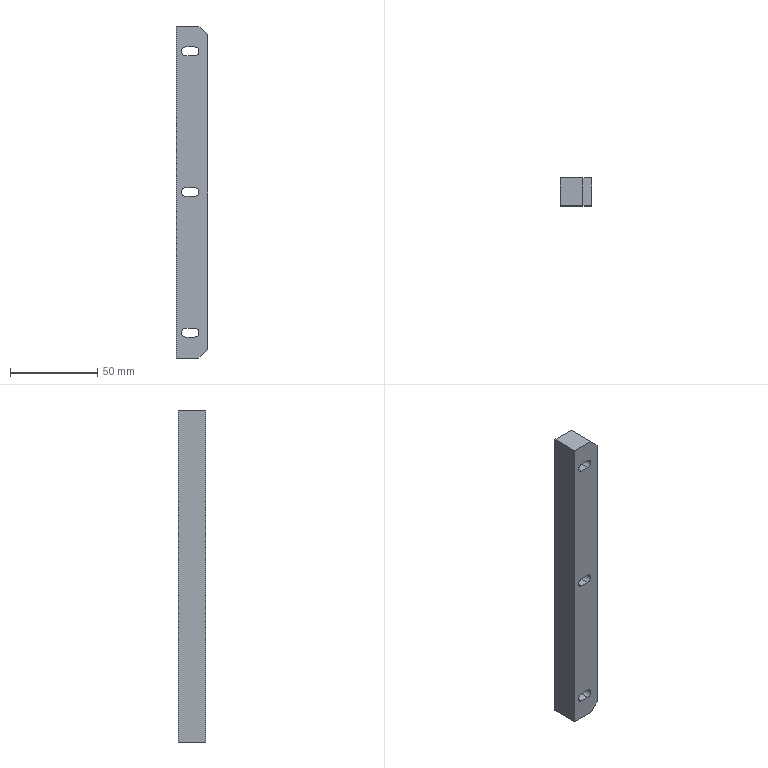Part | SolidWorks | features Chamfer 1, Extrusion 1, ICE 1 | 1 solid | 23 faces | box 18 x 16 x 190 mm | volume 52178 mm3 | plane 14 | cylinder 9 | commonest cylinder face diameters 5 x9
STEP:
#1=CARTESIAN_POINT('',(10.5,16.,83.));
#2=VERTEX_POINT('',#1);
#3=CARTESIAN_POINT('',(13.,16.,80.5));
#4=VERTEX_POINT('',#3);
#5=CARTESIAN_POINT('',(10.5,16.,80.5));
#6=DIRECTION('',(0.,1.,0.));
#7=DIRECTION('',(0.,0.,-1.));
#8=AXIS2_PLACEMENT_3D('',#5,#6,#7);
#9=CIRCLE('',#8,2.5);
#10=EDGE_CURVE('',#2,#4,#9,.T.);
#11=ORIENTED_EDGE('',*,*,#10,.T.);
#12=CARTESIAN_POINT('',(13.,0.,80.5));
#13=VERTEX_POINT('',#12);
#14=CARTESIAN_POINT('',(13.,16.001,80.5));
#15=DIRECTION('',(0.,-1.,0.));
#16=VECTOR('',#15,1000.);
#17=LINE('',#14,#16);
#18=EDGE_CURVE('',#4,#13,#17,.T.);
#19=ORIENTED_EDGE('',*,*,#18,.T.);
#20=CARTESIAN_POINT('',(10.5,0.,83.));
#21=VERTEX_POINT('',#20);
#22=CARTESIAN_POINT('',(10.5,0.,80.5));
#23=DIRECTION('',(0.,-1.,0.));
#24=DIRECTION('',(1.,0.,0.));
#25=AXIS2_PLACEMENT_3D('',#22,#23,#24);
#26=CIRCLE('',#25,2.5);
#27=EDGE_CURVE('',#13,#21,#26,.T.);
#28=ORIENTED_EDGE('',*,*,#27,.T.);
#29=CARTESIAN_POINT('',(10.5,16.001,83.));
#30=DIRECTION('',(0.,-1.,0.));
#31=VECTOR('',#30,1000.);
#32=LINE('',#29,#31);
#33=EDGE_CURVE('',#2,#21,#32,.T.);
#34=ORIENTED_EDGE('',*,*,#33,.F.);
#35=EDGE_LOOP('',(#11,#19,#28,#34));
#36=FACE_OUTER_BOUND('',#35,.T.);
#37=CARTESIAN_POINT('',(10.5,16.001,80.5));
#38=DIRECTION('',(0.,-1.,0.));
#39=DIRECTION('',(1.,0.,0.));
#40=AXIS2_PLACEMENT_3D('',#37,#38,#39);
#41=CYLINDRICAL_SURFACE('',#40,2.5);
#42=ADVANCED_FACE('',(#36),#41,.F.);
#43=CARTESIAN_POINT('',(10.5,16.,2.5));
#44=VERTEX_POINT('',#43);
#45=CARTESIAN_POINT('',(13.,16.,0.));
#46=VERTEX_POINT('',#45);
#47=CARTESIAN_POINT('',(10.5,16.,0.));
#48=DIRECTION('',(0.,1.,0.));
#49=DIRECTION('',(0.,0.,-1.));
#50=AXIS2_PLACEMENT_3D('',#47,#48,#49);
#51=CIRCLE('',#50,2.5);
#52=EDGE_CURVE('',#44,#46,#51,.T.);
#53=ORIENTED_EDGE('',*,*,#52,.T.);
#54=CARTESIAN_POINT('',(13.,0.,0.));
#55=VERTEX_POINT('',#54);
#56=CARTESIAN_POINT('',(13.,16.001,0.));
#57=DIRECTION('',(0.,-1.,0.));
#58=VECTOR('',#57,1000.);
#59=LINE('',#56,#58);
#60=EDGE_CURVE('',#46,#55,#59,.T.);
#61=ORIENTED_EDGE('',*,*,#60,.T.);
#62=CARTESIAN_POINT('',(10.5,0.,2.5));
#63=VERTEX_POINT('',#62);
#64=CARTESIAN_POINT('',(10.5,0.,0.));
#65=DIRECTION('',(0.,-1.,0.));
#66=DIRECTION('',(1.,0.,0.));
#67=AXIS2_PLACEMENT_3D('',#64,#65,#66);
#68=CIRCLE('',#67,2.5);
#69=EDGE_CURVE('',#55,#63,#68,.T.);
#70=ORIENTED_EDGE('',*,*,#69,.T.);
#71=CARTESIAN_POINT('',(10.5,16.001,2.5));
#72=DIRECTION('',(0.,-1.,0.));
#73=VECTOR('',#72,1000.);
#74=LINE('',#71,#73);
#75=EDGE_CURVE('',#44,#63,#74,.T.);
#76=ORIENTED_EDGE('',*,*,#75,.F.);
#77=EDGE_LOOP('',(#53,#61,#70,#76));
#78=FACE_OUTER_BOUND('',#77,.T.);
#79=CARTESIAN_POINT('',(10.5,16.001,0.));
#80=DIRECTION('',(0.,-1.,0.));
#81=DIRECTION('',(1.,0.,0.));
#82=AXIS2_PLACEMENT_3D('',#79,#80,#81);
#83=CYLINDRICAL_SURFACE('',#82,2.5);
#84=ADVANCED_FACE('',(#78),#83,.F.);
#85=CARTESIAN_POINT('',(10.5,16.,-78.));
#86=VERTEX_POINT('',#85);
#87=CARTESIAN_POINT('',(13.,16.,-80.5));
#88=VERTEX_POINT('',#87);
#89=CARTESIAN_POINT('',(10.5,16.,-80.5));
#90=DIRECTION('',(0.,1.,0.));
#91=DIRECTION('',(0.,0.,-1.));
#92=AXIS2_PLACEMENT_3D('',#89,#90,#91);
#93=CIRCLE('',#92,2.5);
#94=EDGE_CURVE('',#86,#88,#93,.T.);
#95=ORIENTED_EDGE('',*,*,#94,.T.);
#96=CARTESIAN_POINT('',(13.,0.,-80.5));
#97=VERTEX_POINT('',#96);
#98=CARTESIAN_POINT('',(13.,16.001,-80.5));
#99=DIRECTION('',(0.,-1.,0.));
#100=VECTOR('',#99,1000.);
#101=LINE('',#98,#100);
#102=EDGE_CURVE('',#88,#97,#101,.T.);
#103=ORIENTED_EDGE('',*,*,#102,.T.);
#104=CARTESIAN_POINT('',(10.5,0.,-78.));
#105=VERTEX_POINT('',#104);
#106=CARTESIAN_POINT('',(10.5,0.,-80.5));
#107=DIRECTION('',(0.,-1.,0.));
#108=DIRECTION('',(-1.,0.,0.));
#109=AXIS2_PLACEMENT_3D('',#106,#107,#108);
#110=CIRCLE('',#109,2.5);
#111=EDGE_CURVE('',#97,#105,#110,.T.);
#112=ORIENTED_EDGE('',*,*,#111,.T.);
#113=CARTESIAN_POINT('',(10.5,16.001,-78.));
#114=DIRECTION('',(0.,-1.,0.));
#115=VECTOR('',#114,1000.);
#116=LINE('',#113,#115);
#117=EDGE_CURVE('',#86,#105,#116,.T.);
#118=ORIENTED_EDGE('',*,*,#117,.F.);
#119=EDGE_LOOP('',(#95,#103,#112,#118));
#120=FACE_OUTER_BOUND('',#119,.T.);
#121=CARTESIAN_POINT('',(10.5,16.001,-80.5));
#122=DIRECTION('',(0.,-1.,0.));
#123=DIRECTION('',(1.,0.,0.));
#124=AXIS2_PLACEMENT_3D('',#121,#122,#123);
#125=CYLINDRICAL_SURFACE('',#124,2.5);
#126=ADVANCED_FACE('',(#120),#125,.F.);
#127=CARTESIAN_POINT('',(5.5,0.,78.));
#128=VERTEX_POINT('',#127);
#129=CARTESIAN_POINT('',(10.5,0.,78.));
#130=VERTEX_POINT('',#129);
#131=CARTESIAN_POINT('',(5.5,0.,78.));
#132=DIRECTION('',(1.,0.,0.));
#133=VECTOR('',#132,1000.);
#134=LINE('',#131,#133);
#135=EDGE_CURVE('',#128,#130,#134,.T.);
#136=ORIENTED_EDGE('',*,*,#135,.F.);
#137=CARTESIAN_POINT('',(5.5,0.,83.));
#138=VERTEX_POINT('',#137);
#139=CARTESIAN_POINT('',(5.5,0.,80.5));
#140=DIRECTION('',(0.,-1.,0.));
#141=DIRECTION('',(1.,0.,0.));
#142=AXIS2_PLACEMENT_3D('',#139,#140,#141);
#143=CIRCLE('',#142,2.5);
#144=EDGE_CURVE('',#138,#128,#143,.T.);
#145=ORIENTED_EDGE('',*,*,#144,.F.);
#146=CARTESIAN_POINT('',(5.5,0.,83.));
#147=DIRECTION('',(-1.,0.,0.));
#148=VECTOR('',#147,1000.);
#149=LINE('',#146,#148);
#150=EDGE_CURVE('',#21,#138,#149,.T.);
#151=ORIENTED_EDGE('',*,*,#150,.F.);
#152=ORIENTED_EDGE('',*,*,#27,.F.);
#153=CARTESIAN_POINT('',(10.5,0.,80.5));
#154=DIRECTION('',(0.,-1.,0.));
#155=DIRECTION('',(1.,0.,0.));
#156=AXIS2_PLACEMENT_3D('',#153,#154,#155);
#157=CIRCLE('',#156,2.5);
#158=EDGE_CURVE('',#130,#13,#157,.T.);
#159=ORIENTED_EDGE('',*,*,#158,.F.);
#160=EDGE_LOOP('',(#136,#145,#151,#152,#159));
#161=FACE_BOUND('',#160,.T.);
#162=CARTESIAN_POINT('',(5.5,0.,-2.5));
#163=VERTEX_POINT('',#162);
#164=CARTESIAN_POINT('',(10.5,0.,-2.5));
#165=VERTEX_POINT('',#164);
#166=CARTESIAN_POINT('',(5.5,0.,-2.5));
#167=DIRECTION('',(1.,0.,0.));
#168=VECTOR('',#167,1000.);
#169=LINE('',#166,#168);
#170=EDGE_CURVE('',#163,#165,#169,.T.);
#171=ORIENTED_EDGE('',*,*,#170,.F.);
#172=CARTESIAN_POINT('',(5.5,0.,2.5));
#173=VERTEX_POINT('',#172);
#174=CARTESIAN_POINT('',(5.5,0.,0.));
#175=DIRECTION('',(0.,-1.,0.));
#176=DIRECTION('',(1.,0.,0.));
#177=AXIS2_PLACEMENT_3D('',#174,#175,#176);
#178=CIRCLE('',#177,2.5);
#179=EDGE_CURVE('',#173,#163,#178,.T.);
#180=ORIENTED_EDGE('',*,*,#179,.F.);
#181=CARTESIAN_POINT('',(5.5,0.,2.5));
#182=DIRECTION('',(-1.,0.,0.));
#183=VECTOR('',#182,1000.);
#184=LINE('',#181,#183);
#185=EDGE_CURVE('',#63,#173,#184,.T.);
#186=ORIENTED_EDGE('',*,*,#185,.F.);
#187=ORIENTED_EDGE('',*,*,#69,.F.);
#188=CARTESIAN_POINT('',(10.5,0.,0.));
#189=DIRECTION('',(0.,-1.,0.));
#190=DIRECTION('',(1.,0.,0.));
#191=AXIS2_PLACEMENT_3D('',#188,#189,#190);
#192=CIRCLE('',#191,2.5);
#193=EDGE_CURVE('',#165,#55,#192,.T.);
#194=ORIENTED_EDGE('',*,*,#193,.F.);
#195=EDGE_LOOP('',(#171,#180,#186,#187,#194));
#196=FACE_BOUND('',#195,.T.);
#197=CARTESIAN_POINT('',(5.5,0.,-83.));
#198=VERTEX_POINT('',#197);
#199=CARTESIAN_POINT('',(10.5,0.,-83.));
#200=VERTEX_POINT('',#199);
#201=CARTESIAN_POINT('',(5.5,0.,-83.));
#202=DIRECTION('',(1.,0.,0.));
#203=VECTOR('',#202,1000.);
#204=LINE('',#201,#203);
#205=EDGE_CURVE('',#198,#200,#204,.T.);
#206=ORIENTED_EDGE('',*,*,#205,.F.);
#207=CARTESIAN_POINT('',(5.5,0.,-78.));
#208=VERTEX_POINT('',#207);
#209=CARTESIAN_POINT('',(5.5,0.,-80.5));
#210=DIRECTION('',(0.,-1.,0.));
#211=DIRECTION('',(-1.,0.,0.));
#212=AXIS2_PLACEMENT_3D('',#209,#210,#211);
#213=CIRCLE('',#212,2.5);
#214=EDGE_CURVE('',#208,#198,#213,.T.);
#215=ORIENTED_EDGE('',*,*,#214,.F.);
#216=CARTESIAN_POINT('',(5.5,0.,-78.));
#217=DIRECTION('',(-1.,0.,0.));
#218=VECTOR('',#217,1000.);
#219=LINE('',#216,#218);
#220=EDGE_CURVE('',#105,#208,#219,.T.);
#221=ORIENTED_EDGE('',*,*,#220,.F.);
#222=ORIENTED_EDGE('',*,*,#111,.F.);
#223=CARTESIAN_POINT('',(10.5,0.,-80.5));
#224=DIRECTION('',(0.,-1.,0.));
#225=DIRECTION('',(-1.,0.,0.));
#226=AXIS2_PLACEMENT_3D('',#223,#224,#225);
#227=CIRCLE('',#226,2.5);
#228=EDGE_CURVE('',#200,#97,#227,.T.);
#229=ORIENTED_EDGE('',*,*,#228,.F.);
#230=EDGE_LOOP('',(#206,#215,#221,#222,#229));
#231=FACE_BOUND('',#230,.T.);
#232=CARTESIAN_POINT('',(0.,0.,-95.));
#233=VERTEX_POINT('',#232);
#234=CARTESIAN_POINT('',(13.,0.,-95.));
#235=VERTEX_POINT('',#234);
#236=CARTESIAN_POINT('',(18.,0.,-95.));
#237=DIRECTION('',(1.,0.,0.));
#238=VECTOR('',#237,1000.);
#239=LINE('',#236,#238);
#240=EDGE_CURVE('',#233,#235,#239,.T.);
#241=ORIENTED_EDGE('',*,*,#240,.T.);
#242=CARTESIAN_POINT('',(18.,0.,-90.));
#243=VERTEX_POINT('',#242);
#244=CARTESIAN_POINT('',(18.,0.,-90.));
#245=DIRECTION('',(0.7071,0.,0.7071));
#246=VECTOR('',#245,1000.);
#247=LINE('',#244,#246);
#248=EDGE_CURVE('',#235,#243,#247,.T.);
#249=ORIENTED_EDGE('',*,*,#248,.T.);
#250=CARTESIAN_POINT('',(18.,0.,90.));
#251=VERTEX_POINT('',#250);
#252=CARTESIAN_POINT('',(18.,0.,95.));
#253=DIRECTION('',(0.,0.,-1.));
#254=VECTOR('',#253,1000.);
#255=LINE('',#252,#254);
#256=EDGE_CURVE('',#251,#243,#255,.T.);
#257=ORIENTED_EDGE('',*,*,#256,.F.);
#258=CARTESIAN_POINT('',(13.,0.,95.));
#259=VERTEX_POINT('',#258);
#260=CARTESIAN_POINT('',(13.,0.,95.));
#261=DIRECTION('',(-0.7071,0.,0.7071));
#262=VECTOR('',#261,1000.);
#263=LINE('',#260,#262);
#264=EDGE_CURVE('',#251,#259,#263,.T.);
#265=ORIENTED_EDGE('',*,*,#264,.T.);
#266=CARTESIAN_POINT('',(0.,0.,95.));
#267=VERTEX_POINT('',#266);
#268=CARTESIAN_POINT('',(18.,0.,95.));
#269=DIRECTION('',(1.,0.,0.));
#270=VECTOR('',#269,1000.);
#271=LINE('',#268,#270);
#272=EDGE_CURVE('',#267,#259,#271,.T.);
#273=ORIENTED_EDGE('',*,*,#272,.F.);
#274=CARTESIAN_POINT('',(0.,0.,95.));
#275=DIRECTION('',(0.,0.,-1.));
#276=VECTOR('',#275,1000.);
#277=LINE('',#274,#276);
#278=EDGE_CURVE('',#267,#233,#277,.T.);
#279=ORIENTED_EDGE('',*,*,#278,.T.);
#280=EDGE_LOOP('',(#241,#249,#257,#265,#273,#279));
#281=FACE_OUTER_BOUND('',#280,.T.);
#282=CARTESIAN_POINT('',(18.,0.,95.));
#283=DIRECTION('',(0.,1.,0.));
#284=DIRECTION('',(-1.,0.,0.));
#285=AXIS2_PLACEMENT_3D('',#282,#283,#284);
#286=PLANE('',#285);
#287=ADVANCED_FACE('',(#161,#196,#231,#281),#286,.F.);
#288=ORIENTED_EDGE('',*,*,#256,.T.);
#289=CARTESIAN_POINT('',(18.,16.,-90.));
#290=VERTEX_POINT('',#289);
#291=CARTESIAN_POINT('',(18.,16.,-90.));
#292=DIRECTION('',(0.,1.,0.));
#293=VECTOR('',#292,1000.);
#294=LINE('',#291,#293);
#295=EDGE_CURVE('',#243,#290,#294,.T.);
#296=ORIENTED_EDGE('',*,*,#295,.T.);
#297=CARTESIAN_POINT('',(18.,16.,90.));
#298=VERTEX_POINT('',#297);
#299=CARTESIAN_POINT('',(18.,16.,95.));
#300=DIRECTION('',(0.,0.,-1.));
#301=VECTOR('',#300,1000.);
#302=LINE('',#299,#301);
#303=EDGE_CURVE('',#298,#290,#302,.T.);
#304=ORIENTED_EDGE('',*,*,#303,.F.);
#305=CARTESIAN_POINT('',(18.,16.,90.));
#306=DIRECTION('',(0.,-1.,0.));
#307=VECTOR('',#306,1000.);
#308=LINE('',#305,#307);
#309=EDGE_CURVE('',#298,#251,#308,.T.);
#310=ORIENTED_EDGE('',*,*,#309,.T.);
#311=EDGE_LOOP('',(#288,#296,#304,#310));
#312=FACE_OUTER_BOUND('',#311,.T.);
#313=CARTESIAN_POINT('',(18.,16.,95.));
#314=DIRECTION('',(-1.,0.,0.));
#315=DIRECTION('',(0.,-1.,0.));
#316=AXIS2_PLACEMENT_3D('',#313,#314,#315);
#317=PLANE('',#316);
#318=ADVANCED_FACE('',(#312),#317,.F.);
#319=CARTESIAN_POINT('',(5.5,16.,83.));
#320=VERTEX_POINT('',#319);
#321=CARTESIAN_POINT('',(5.5,16.,83.));
#322=DIRECTION('',(1.,0.,0.));
#323=VECTOR('',#322,1000.);
#324=LINE('',#321,#323);
#325=EDGE_CURVE('',#320,#2,#324,.T.);
#326=ORIENTED_EDGE('',*,*,#325,.F.);
#327=CARTESIAN_POINT('',(5.5,16.,78.));
#328=VERTEX_POINT('',#327);
#329=CARTESIAN_POINT('',(5.5,16.,80.5));
#330=DIRECTION('',(0.,1.,0.));
#331=DIRECTION('',(0.,0.,-1.));
#332=AXIS2_PLACEMENT_3D('',#329,#330,#331);
#333=CIRCLE('',#332,2.5);
#334=EDGE_CURVE('',#328,#320,#333,.T.);
#335=ORIENTED_EDGE('',*,*,#334,.F.);
#336=CARTESIAN_POINT('',(10.5,16.,78.));
#337=VERTEX_POINT('',#336);
#338=CARTESIAN_POINT('',(5.5,16.,78.));
#339=DIRECTION('',(-1.,0.,0.));
#340=VECTOR('',#339,1000.);
#341=LINE('',#338,#340);
#342=EDGE_CURVE('',#337,#328,#341,.T.);
#343=ORIENTED_EDGE('',*,*,#342,.F.);
#344=CARTESIAN_POINT('',(10.5,16.,80.5));
#345=DIRECTION('',(0.,1.,0.));
#346=DIRECTION('',(0.,0.,-1.));
#347=AXIS2_PLACEMENT_3D('',#344,#345,#346);
#348=CIRCLE('',#347,2.5);
#349=EDGE_CURVE('',#4,#337,#348,.T.);
#350=ORIENTED_EDGE('',*,*,#349,.F.);
#351=ORIENTED_EDGE('',*,*,#10,.F.);
#352=EDGE_LOOP('',(#326,#335,#343,#350,#351));
#353=FACE_BOUND('',#352,.T.);
#354=CARTESIAN_POINT('',(5.5,16.,2.5));
#355=VERTEX_POINT('',#354);
#356=CARTESIAN_POINT('',(5.5,16.,2.5));
#357=DIRECTION('',(1.,0.,0.));
#358=VECTOR('',#357,1000.);
#359=LINE('',#356,#358);
#360=EDGE_CURVE('',#355,#44,#359,.T.);
#361=ORIENTED_EDGE('',*,*,#360,.F.);
#362=CARTESIAN_POINT('',(5.5,16.,-2.5));
#363=VERTEX_POINT('',#362);
#364=CARTESIAN_POINT('',(5.5,16.,0.));
#365=DIRECTION('',(0.,1.,0.));
#366=DIRECTION('',(0.,0.,-1.));
#367=AXIS2_PLACEMENT_3D('',#364,#365,#366);
#368=CIRCLE('',#367,2.5);
#369=EDGE_CURVE('',#363,#355,#368,.T.);
#370=ORIENTED_EDGE('',*,*,#369,.F.);
#371=CARTESIAN_POINT('',(10.5,16.,-2.5));
#372=VERTEX_POINT('',#371);
#373=CARTESIAN_POINT('',(5.5,16.,-2.5));
#374=DIRECTION('',(-1.,0.,0.));
#375=VECTOR('',#374,1000.);
#376=LINE('',#373,#375);
#377=EDGE_CURVE('',#372,#363,#376,.T.);
#378=ORIENTED_EDGE('',*,*,#377,.F.);
#379=CARTESIAN_POINT('',(10.5,16.,0.));
#380=DIRECTION('',(0.,1.,0.));
#381=DIRECTION('',(0.,0.,-1.));
#382=AXIS2_PLACEMENT_3D('',#379,#380,#381);
#383=CIRCLE('',#382,2.5);
#384=EDGE_CURVE('',#46,#372,#383,.T.);
#385=ORIENTED_EDGE('',*,*,#384,.F.);
#386=ORIENTED_EDGE('',*,*,#52,.F.);
#387=EDGE_LOOP('',(#361,#370,#378,#385,#386));
#388=FACE_BOUND('',#387,.T.);
#389=CARTESIAN_POINT('',(5.5,16.,-78.));
#390=VERTEX_POINT('',#389);
#391=CARTESIAN_POINT('',(5.5,16.,-78.));
#392=DIRECTION('',(1.,0.,0.));
#393=VECTOR('',#392,1000.);
#394=LINE('',#391,#393);
#395=EDGE_CURVE('',#390,#86,#394,.T.);
#396=ORIENTED_EDGE('',*,*,#395,.F.);
#397=CARTESIAN_POINT('',(5.5,16.,-83.));
#398=VERTEX_POINT('',#397);
#399=CARTESIAN_POINT('',(5.5,16.,-80.5));
#400=DIRECTION('',(0.,1.,0.));
#401=DIRECTION('',(0.,0.,-1.));
#402=AXIS2_PLACEMENT_3D('',#399,#400,#401);
#403=CIRCLE('',#402,2.5);
#404=EDGE_CURVE('',#398,#390,#403,.T.);
#405=ORIENTED_EDGE('',*,*,#404,.F.);
#406=CARTESIAN_POINT('',(10.5,16.,-83.));
#407=VERTEX_POINT('',#406);
#408=CARTESIAN_POINT('',(5.5,16.,-83.));
#409=DIRECTION('',(-1.,0.,0.));
#410=VECTOR('',#409,1000.);
#411=LINE('',#408,#410);
#412=EDGE_CURVE('',#407,#398,#411,.T.);
#413=ORIENTED_EDGE('',*,*,#412,.F.);
#414=CARTESIAN_POINT('',(10.5,16.,-80.5));
#415=DIRECTION('',(0.,1.,0.));
#416=DIRECTION('',(0.,0.,-1.));
#417=AXIS2_PLACEMENT_3D('',#414,#415,#416);
#418=CIRCLE('',#417,2.5);
#419=EDGE_CURVE('',#88,#407,#418,.T.);
#420=ORIENTED_EDGE('',*,*,#419,.F.);
#421=ORIENTED_EDGE('',*,*,#94,.F.);
#422=EDGE_LOOP('',(#396,#405,#413,#420,#421));
#423=FACE_BOUND('',#422,.T.);
#424=ORIENTED_EDGE('',*,*,#303,.T.);
#425=CARTESIAN_POINT('',(13.,16.,-95.));
#426=VERTEX_POINT('',#425);
#427=CARTESIAN_POINT('',(18.,16.,-90.));
#428=DIRECTION('',(-0.7071,0.,-0.7071));
#429=VECTOR('',#428,1000.);
#430=LINE('',#427,#429);
#431=EDGE_CURVE('',#290,#426,#430,.T.);
#432=ORIENTED_EDGE('',*,*,#431,.T.);
#433=CARTESIAN_POINT('',(0.,16.,-95.));
#434=VERTEX_POINT('',#433);
#435=CARTESIAN_POINT('',(0.,16.,-95.));
#436=DIRECTION('',(-1.,0.,0.));
#437=VECTOR('',#436,1000.);
#438=LINE('',#435,#437);
#439=EDGE_CURVE('',#426,#434,#438,.T.);
#440=ORIENTED_EDGE('',*,*,#439,.T.);
#441=CARTESIAN_POINT('',(0.,16.,95.));
#442=VERTEX_POINT('',#441);
#443=CARTESIAN_POINT('',(0.,16.,95.));
#444=DIRECTION('',(0.,0.,-1.));
#445=VECTOR('',#444,1000.);
#446=LINE('',#443,#445);
#447=EDGE_CURVE('',#442,#434,#446,.T.);
#448=ORIENTED_EDGE('',*,*,#447,.F.);
#449=CARTESIAN_POINT('',(13.,16.,95.));
#450=VERTEX_POINT('',#449);
#451=CARTESIAN_POINT('',(0.,16.,95.));
#452=DIRECTION('',(-1.,0.,0.));
#453=VECTOR('',#452,1000.);
#454=LINE('',#451,#453);
#455=EDGE_CURVE('',#450,#442,#454,.T.);
#456=ORIENTED_EDGE('',*,*,#455,.F.);
#457=CARTESIAN_POINT('',(13.,16.,95.));
#458=DIRECTION('',(0.7071,0.,-0.7071));
#459=VECTOR('',#458,1000.);
#460=LINE('',#457,#459);
#461=EDGE_CURVE('',#450,#298,#460,.T.);
#462=ORIENTED_EDGE('',*,*,#461,.T.);
#463=EDGE_LOOP('',(#424,#432,#440,#448,#456,#462));
#464=FACE_OUTER_BOUND('',#463,.T.);
#465=CARTESIAN_POINT('',(0.,16.,95.));
#466=DIRECTION('',(0.,-1.,0.));
#467=DIRECTION('',(0.,0.,-1.));
#468=AXIS2_PLACEMENT_3D('',#465,#466,#467);
#469=PLANE('',#468);
#470=ADVANCED_FACE('',(#353,#388,#423,#464),#469,.F.);
#471=CARTESIAN_POINT('',(0.,0.,-95.));
#472=DIRECTION('',(0.,-1.,0.));
#473=VECTOR('',#472,1000.);
#474=LINE('',#471,#473);
#475=EDGE_CURVE('',#434,#233,#474,.T.);
#476=ORIENTED_EDGE('',*,*,#475,.T.);
#477=ORIENTED_EDGE('',*,*,#278,.F.);
#478=CARTESIAN_POINT('',(0.,0.,95.));
#479=DIRECTION('',(0.,-1.,0.));
#480=VECTOR('',#479,1000.);
#481=LINE('',#478,#480);
#482=EDGE_CURVE('',#442,#267,#481,.T.);
#483=ORIENTED_EDGE('',*,*,#482,.F.);
#484=ORIENTED_EDGE('',*,*,#447,.T.);
#485=EDGE_LOOP('',(#476,#477,#483,#484));
#486=FACE_OUTER_BOUND('',#485,.T.);
#487=CARTESIAN_POINT('',(0.,0.,95.));
#488=DIRECTION('',(1.,0.,0.));
#489=DIRECTION('',(0.,0.,-1.));
#490=AXIS2_PLACEMENT_3D('',#487,#488,#489);
#491=PLANE('',#490);
#492=ADVANCED_FACE('',(#486),#491,.F.);
#493=ORIENTED_EDGE('',*,*,#272,.T.);
#494=CARTESIAN_POINT('',(13.,0.,95.));
#495=DIRECTION('',(0.,1.,0.));
#496=VECTOR('',#495,1000.);
#497=LINE('',#494,#496);
#498=EDGE_CURVE('',#259,#450,#497,.T.);
#499=ORIENTED_EDGE('',*,*,#498,.T.);
#500=ORIENTED_EDGE('',*,*,#455,.T.);
#501=ORIENTED_EDGE('',*,*,#482,.T.);
#502=EDGE_LOOP('',(#493,#499,#500,#501));
#503=FACE_OUTER_BOUND('',#502,.T.);
#504=CARTESIAN_POINT('',(0.,0.,95.));
#505=DIRECTION('',(0.,0.,-1.));
#506=DIRECTION('',(-1.,0.,0.));
#507=AXIS2_PLACEMENT_3D('',#504,#505,#506);
#508=PLANE('',#507);
#509=ADVANCED_FACE('',(#503),#508,.F.);
#510=ORIENTED_EDGE('',*,*,#439,.F.);
#511=CARTESIAN_POINT('',(13.,0.,-95.));
#512=DIRECTION('',(0.,-1.,0.));
#513=VECTOR('',#512,1000.);
#514=LINE('',#511,#513);
#515=EDGE_CURVE('',#426,#235,#514,.T.);
#516=ORIENTED_EDGE('',*,*,#515,.T.);
#517=ORIENTED_EDGE('',*,*,#240,.F.);
#518=ORIENTED_EDGE('',*,*,#475,.F.);
#519=EDGE_LOOP('',(#510,#516,#517,#518));
#520=FACE_OUTER_BOUND('',#519,.T.);
#521=CARTESIAN_POINT('',(0.,0.,-95.));
#522=DIRECTION('',(0.,0.,-1.));
#523=DIRECTION('',(-1.,0.,0.));
#524=AXIS2_PLACEMENT_3D('',#521,#522,#523);
#525=PLANE('',#524);
#526=ADVANCED_FACE('',(#520),#525,.T.);
#527=ORIENTED_EDGE('',*,*,#248,.F.);
#528=ORIENTED_EDGE('',*,*,#515,.F.);
#529=ORIENTED_EDGE('',*,*,#431,.F.);
#530=ORIENTED_EDGE('',*,*,#295,.F.);
#531=EDGE_LOOP('',(#527,#528,#529,#530));
#532=FACE_OUTER_BOUND('',#531,.T.);
#533=CARTESIAN_POINT('',(18.,16.,-90.));
#534=DIRECTION('',(0.7071,0.,-0.7071));
#535=DIRECTION('',(0.,-1.,0.));
#536=AXIS2_PLACEMENT_3D('',#533,#534,#535);
#537=PLANE('',#536);
#538=ADVANCED_FACE('',(#532),#537,.T.);
#539=ORIENTED_EDGE('',*,*,#264,.F.);
#540=ORIENTED_EDGE('',*,*,#309,.F.);
#541=ORIENTED_EDGE('',*,*,#461,.F.);
#542=ORIENTED_EDGE('',*,*,#498,.F.);
#543=EDGE_LOOP('',(#539,#540,#541,#542));
#544=FACE_OUTER_BOUND('',#543,.T.);
#545=CARTESIAN_POINT('',(13.,0.,95.));
#546=DIRECTION('',(-0.7071,0.,-0.7071));
#547=DIRECTION('',(0.,1.,0.));
#548=AXIS2_PLACEMENT_3D('',#545,#546,#547);
#549=PLANE('',#548);
#550=ADVANCED_FACE('',(#544),#549,.F.);
#551=ORIENTED_EDGE('',*,*,#404,.T.);
#552=CARTESIAN_POINT('',(5.5,16.001,-78.));
#553=DIRECTION('',(0.,-1.,0.));
#554=VECTOR('',#553,1000.);
#555=LINE('',#552,#554);
#556=EDGE_CURVE('',#390,#208,#555,.T.);
#557=ORIENTED_EDGE('',*,*,#556,.T.);
#558=ORIENTED_EDGE('',*,*,#214,.T.);
#559=CARTESIAN_POINT('',(5.5,16.001,-83.));
#560=DIRECTION('',(0.,-1.,0.));
#561=VECTOR('',#560,1000.);
#562=LINE('',#559,#561);
#563=EDGE_CURVE('',#398,#198,#562,.T.);
#564=ORIENTED_EDGE('',*,*,#563,.F.);
#565=EDGE_LOOP('',(#551,#557,#558,#564));
#566=FACE_OUTER_BOUND('',#565,.T.);
#567=CARTESIAN_POINT('',(5.5,16.001,-80.5));
#568=DIRECTION('',(0.,-1.,0.));
#569=DIRECTION('',(1.,0.,0.));
#570=AXIS2_PLACEMENT_3D('',#567,#568,#569);
#571=CYLINDRICAL_SURFACE('',#570,2.5);
#572=ADVANCED_FACE('',(#566),#571,.F.);
#573=ORIENTED_EDGE('',*,*,#395,.T.);
#574=ORIENTED_EDGE('',*,*,#117,.T.);
#575=ORIENTED_EDGE('',*,*,#220,.T.);
#576=ORIENTED_EDGE('',*,*,#556,.F.);
#577=EDGE_LOOP('',(#573,#574,#575,#576));
#578=FACE_OUTER_BOUND('',#577,.T.);
#579=CARTESIAN_POINT('',(5.5,16.001,-78.));
#580=DIRECTION('',(0.,0.,1.));
#581=DIRECTION('',(1.,0.,0.));
#582=AXIS2_PLACEMENT_3D('',#579,#580,#581);
#583=PLANE('',#582);
#584=ADVANCED_FACE('',(#578),#583,.F.);
#585=ORIENTED_EDGE('',*,*,#102,.F.);
#586=ORIENTED_EDGE('',*,*,#419,.T.);
#587=CARTESIAN_POINT('',(10.5,16.001,-83.));
#588=DIRECTION('',(0.,-1.,0.));
#589=VECTOR('',#588,1000.);
#590=LINE('',#587,#589);
#591=EDGE_CURVE('',#407,#200,#590,.T.);
#592=ORIENTED_EDGE('',*,*,#591,.T.);
#593=ORIENTED_EDGE('',*,*,#228,.T.);
#594=EDGE_LOOP('',(#585,#586,#592,#593));
#595=FACE_OUTER_BOUND('',#594,.T.);
#596=CARTESIAN_POINT('',(10.5,16.001,-80.5));
#597=DIRECTION('',(0.,-1.,0.));
#598=DIRECTION('',(1.,0.,0.));
#599=AXIS2_PLACEMENT_3D('',#596,#597,#598);
#600=CYLINDRICAL_SURFACE('',#599,2.5);
#601=ADVANCED_FACE('',(#595),#600,.F.);
#602=ORIENTED_EDGE('',*,*,#412,.T.);
#603=ORIENTED_EDGE('',*,*,#563,.T.);
#604=ORIENTED_EDGE('',*,*,#205,.T.);
#605=ORIENTED_EDGE('',*,*,#591,.F.);
#606=EDGE_LOOP('',(#602,#603,#604,#605));
#607=FACE_OUTER_BOUND('',#606,.T.);
#608=CARTESIAN_POINT('',(5.5,16.001,-83.));
#609=DIRECTION('',(0.,0.,-1.));
#610=DIRECTION('',(-1.,0.,0.));
#611=AXIS2_PLACEMENT_3D('',#608,#609,#610);
#612=PLANE('',#611);
#613=ADVANCED_FACE('',(#607),#612,.F.);
#614=ORIENTED_EDGE('',*,*,#369,.T.);
#615=CARTESIAN_POINT('',(5.5,16.001,2.5));
#616=DIRECTION('',(0.,-1.,0.));
#617=VECTOR('',#616,1000.);
#618=LINE('',#615,#617);
#619=EDGE_CURVE('',#355,#173,#618,.T.);
#620=ORIENTED_EDGE('',*,*,#619,.T.);
#621=ORIENTED_EDGE('',*,*,#179,.T.);
#622=CARTESIAN_POINT('',(5.5,16.001,-2.5));
#623=DIRECTION('',(0.,-1.,0.));
#624=VECTOR('',#623,1000.);
#625=LINE('',#622,#624);
#626=EDGE_CURVE('',#363,#163,#625,.T.);
#627=ORIENTED_EDGE('',*,*,#626,.F.);
#628=EDGE_LOOP('',(#614,#620,#621,#627));
#629=FACE_OUTER_BOUND('',#628,.T.);
#630=CARTESIAN_POINT('',(5.5,16.001,0.));
#631=DIRECTION('',(0.,-1.,0.));
#632=DIRECTION('',(1.,0.,0.));
#633=AXIS2_PLACEMENT_3D('',#630,#631,#632);
#634=CYLINDRICAL_SURFACE('',#633,2.5);
#635=ADVANCED_FACE('',(#629),#634,.F.);
#636=ORIENTED_EDGE('',*,*,#360,.T.);
#637=ORIENTED_EDGE('',*,*,#75,.T.);
#638=ORIENTED_EDGE('',*,*,#185,.T.);
#639=ORIENTED_EDGE('',*,*,#619,.F.);
#640=EDGE_LOOP('',(#636,#637,#638,#639));
#641=FACE_OUTER_BOUND('',#640,.T.);
#642=CARTESIAN_POINT('',(5.5,16.001,2.5));
#643=DIRECTION('',(0.,0.,1.));
#644=DIRECTION('',(1.,0.,0.));
#645=AXIS2_PLACEMENT_3D('',#642,#643,#644);
#646=PLANE('',#645);
#647=ADVANCED_FACE('',(#641),#646,.F.);
#648=ORIENTED_EDGE('',*,*,#60,.F.);
#649=ORIENTED_EDGE('',*,*,#384,.T.);
#650=CARTESIAN_POINT('',(10.5,16.001,-2.5));
#651=DIRECTION('',(0.,-1.,0.));
#652=VECTOR('',#651,1000.);
#653=LINE('',#650,#652);
#654=EDGE_CURVE('',#372,#165,#653,.T.);
#655=ORIENTED_EDGE('',*,*,#654,.T.);
#656=ORIENTED_EDGE('',*,*,#193,.T.);
#657=EDGE_LOOP('',(#648,#649,#655,#656));
#658=FACE_OUTER_BOUND('',#657,.T.);
#659=CARTESIAN_POINT('',(10.5,16.001,0.));
#660=DIRECTION('',(0.,-1.,0.));
#661=DIRECTION('',(1.,0.,0.));
#662=AXIS2_PLACEMENT_3D('',#659,#660,#661);
#663=CYLINDRICAL_SURFACE('',#662,2.5);
#664=ADVANCED_FACE('',(#658),#663,.F.);
#665=ORIENTED_EDGE('',*,*,#377,.T.);
#666=ORIENTED_EDGE('',*,*,#626,.T.);
#667=ORIENTED_EDGE('',*,*,#170,.T.);
#668=ORIENTED_EDGE('',*,*,#654,.F.);
#669=EDGE_LOOP('',(#665,#666,#667,#668));
#670=FACE_OUTER_BOUND('',#669,.T.);
#671=CARTESIAN_POINT('',(5.5,16.001,-2.5));
#672=DIRECTION('',(0.,0.,-1.));
#673=DIRECTION('',(-1.,0.,0.));
#674=AXIS2_PLACEMENT_3D('',#671,#672,#673);
#675=PLANE('',#674);
#676=ADVANCED_FACE('',(#670),#675,.F.);
#677=ORIENTED_EDGE('',*,*,#334,.T.);
#678=CARTESIAN_POINT('',(5.5,16.001,83.));
#679=DIRECTION('',(0.,-1.,0.));
#680=VECTOR('',#679,1000.);
#681=LINE('',#678,#680);
#682=EDGE_CURVE('',#320,#138,#681,.T.);
#683=ORIENTED_EDGE('',*,*,#682,.T.);
#684=ORIENTED_EDGE('',*,*,#144,.T.);
#685=CARTESIAN_POINT('',(5.5,16.001,78.));
#686=DIRECTION('',(0.,-1.,0.));
#687=VECTOR('',#686,1000.);
#688=LINE('',#685,#687);
#689=EDGE_CURVE('',#328,#128,#688,.T.);
#690=ORIENTED_EDGE('',*,*,#689,.F.);
#691=EDGE_LOOP('',(#677,#683,#684,#690));
#692=FACE_OUTER_BOUND('',#691,.T.);
#693=CARTESIAN_POINT('',(5.5,16.001,80.5));
#694=DIRECTION('',(0.,-1.,0.));
#695=DIRECTION('',(1.,0.,0.));
#696=AXIS2_PLACEMENT_3D('',#693,#694,#695);
#697=CYLINDRICAL_SURFACE('',#696,2.5);
#698=ADVANCED_FACE('',(#692),#697,.F.);
#699=ORIENTED_EDGE('',*,*,#325,.T.);
#700=ORIENTED_EDGE('',*,*,#33,.T.);
#701=ORIENTED_EDGE('',*,*,#150,.T.);
#702=ORIENTED_EDGE('',*,*,#682,.F.);
#703=EDGE_LOOP('',(#699,#700,#701,#702));
#704=FACE_OUTER_BOUND('',#703,.T.);
#705=CARTESIAN_POINT('',(5.5,16.001,83.));
#706=DIRECTION('',(0.,0.,1.));
#707=DIRECTION('',(1.,0.,0.));
#708=AXIS2_PLACEMENT_3D('',#705,#706,#707);
#709=PLANE('',#708);
#710=ADVANCED_FACE('',(#704),#709,.F.);
#711=ORIENTED_EDGE('',*,*,#18,.F.);
#712=ORIENTED_EDGE('',*,*,#349,.T.);
#713=CARTESIAN_POINT('',(10.5,16.001,78.));
#714=DIRECTION('',(0.,-1.,0.));
#715=VECTOR('',#714,1000.);
#716=LINE('',#713,#715);
#717=EDGE_CURVE('',#337,#130,#716,.T.);
#718=ORIENTED_EDGE('',*,*,#717,.T.);
#719=ORIENTED_EDGE('',*,*,#158,.T.);
#720=EDGE_LOOP('',(#711,#712,#718,#719));
#721=FACE_OUTER_BOUND('',#720,.T.);
#722=CARTESIAN_POINT('',(10.5,16.001,80.5));
#723=DIRECTION('',(0.,-1.,0.));
#724=DIRECTION('',(1.,0.,0.));
#725=AXIS2_PLACEMENT_3D('',#722,#723,#724);
#726=CYLINDRICAL_SURFACE('',#725,2.5);
#727=ADVANCED_FACE('',(#721),#726,.F.);
#728=ORIENTED_EDGE('',*,*,#342,.T.);
#729=ORIENTED_EDGE('',*,*,#689,.T.);
#730=ORIENTED_EDGE('',*,*,#135,.T.);
#731=ORIENTED_EDGE('',*,*,#717,.F.);
#732=EDGE_LOOP('',(#728,#729,#730,#731));
#733=FACE_OUTER_BOUND('',#732,.T.);
#734=CARTESIAN_POINT('',(5.5,16.001,78.));
#735=DIRECTION('',(0.,0.,-1.));
#736=DIRECTION('',(-1.,0.,0.));
#737=AXIS2_PLACEMENT_3D('',#734,#735,#736);
#738=PLANE('',#737);
#739=ADVANCED_FACE('',(#733),#738,.F.);
#740=CLOSED_SHELL('',(#42,#84,#126,#287,#318,#470,#492,#509,#526,#538,#550,#572,#584,#601,#613,#635,#647,#664,#676,#698,#710,#727,#739));
#741=MANIFOLD_SOLID_BREP('',#740);
#742=CARTESIAN_POINT('',(0.,0.,0.));
#743=DIRECTION('',(0.,0.,1.));
#744=DIRECTION('',(1.,0.,0.));
#745=AXIS2_PLACEMENT_3D('',#742,#743,#744);
#746=(LENGTH_UNIT()NAMED_UNIT(*)SI_UNIT(.MILLI.,.METRE.));
#747=UNCERTAINTY_MEASURE_WITH_UNIT(LENGTH_MEASURE(0.00001),#746,'','');
#748=(NAMED_UNIT(*)PLANE_ANGLE_UNIT()SI_UNIT($,.RADIAN.));
#749=(NAMED_UNIT(*)SI_UNIT($,.STERADIAN.)SOLID_ANGLE_UNIT());
#750=(GEOMETRIC_REPRESENTATION_CONTEXT(3)GLOBAL_UNCERTAINTY_ASSIGNED_CONTEXT((#747))GLOBAL_UNIT_ASSIGNED_CONTEXT((#746,#748,#749))REPRESENTATION_CONTEXT('',''));
#751=ADVANCED_BREP_SHAPE_REPRESENTATION('',(#741,#745),#750);